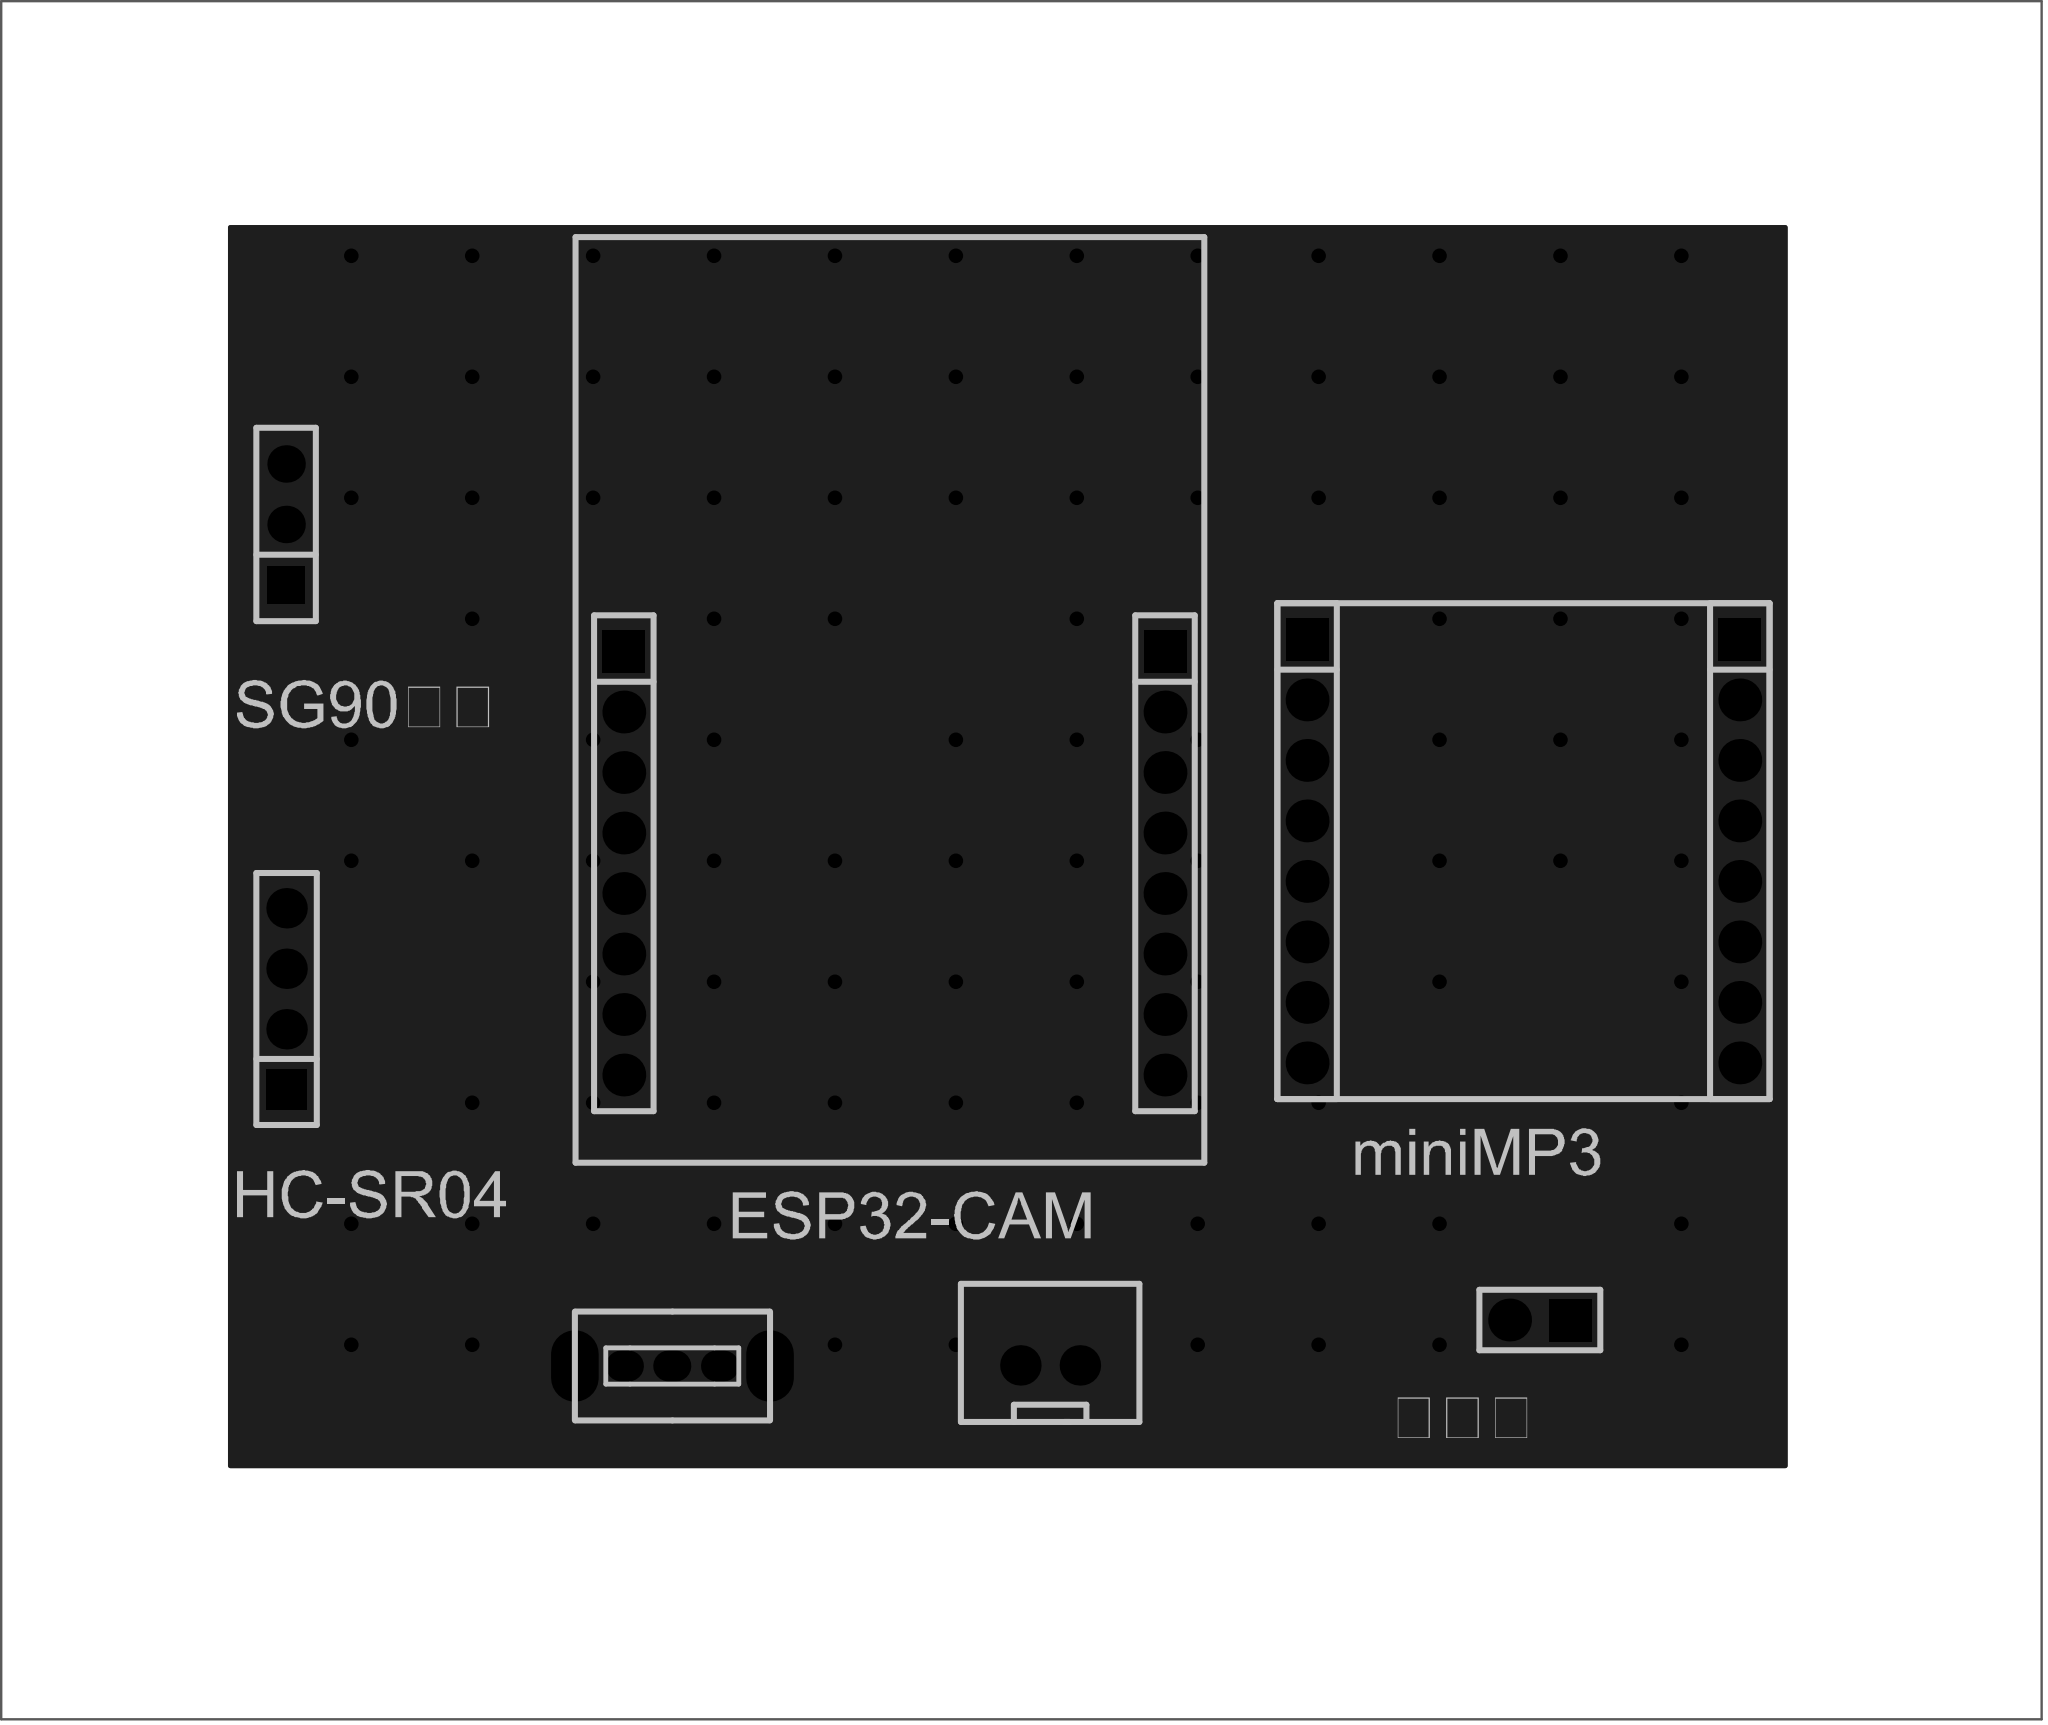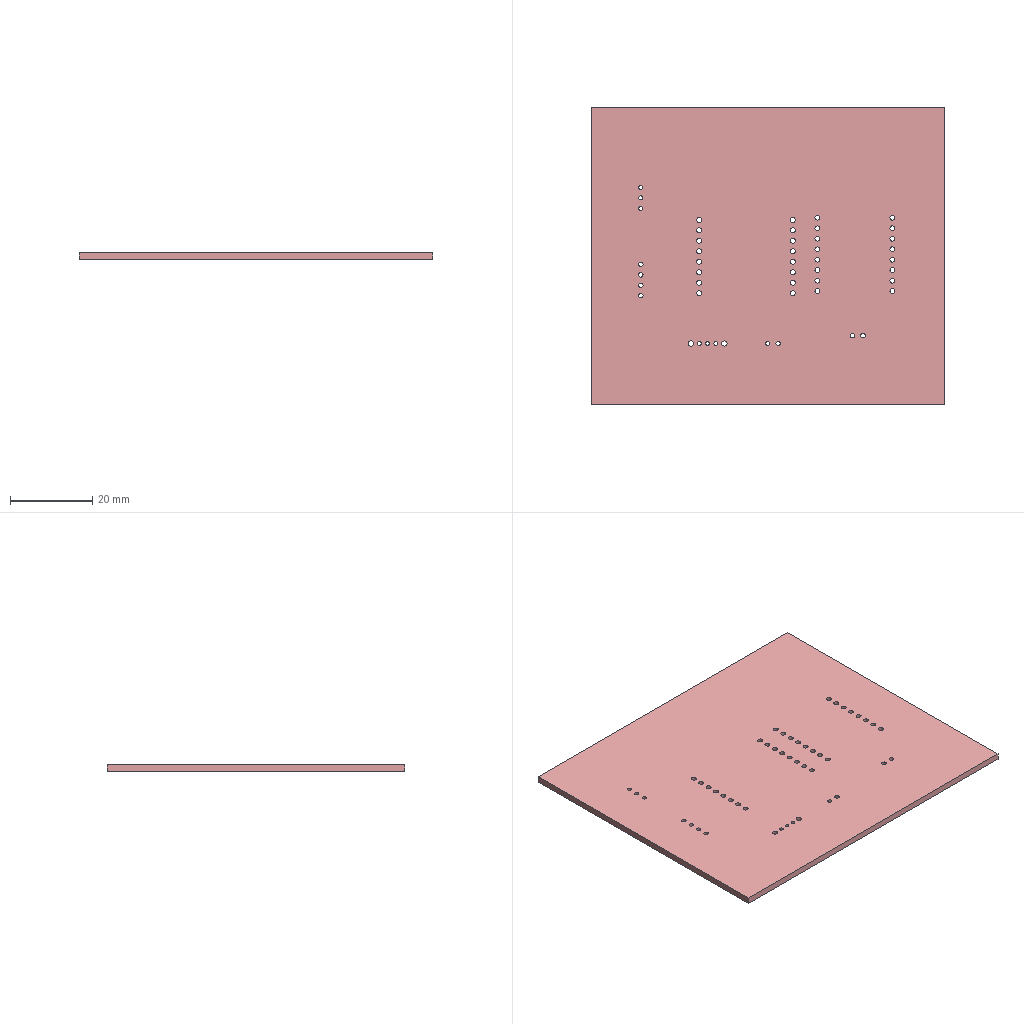Circuit board layout | Altium Designer | box 85.7 x 72.1 x 1.6 mm
Layer stack:
# Altium Designer layer stack of  (unit mm; dielectric type: 0 none, 1 core, 2 prepreg, 3 surface material)
index,name,kind,layer,copper_thickness_mm,dielectric_type,dielectric_thickness_mm,dielectric_material,dielectric_constant
0,Top Paste Mask Layer,other,,,,,,
1,Top Silkscreen Layer,other,,,,,,
2,Top Solder Mask Layer,dielectric,,,3,0.01,,3.3
3,Top Layer,copper,Top Layer,0.035,,,,
4,Dielectric1,dielectric,,,3,1.51,FR4,4.5
5,Bottom Layer,copper,Bottom Layer,0.035,,,,
6,Bottom Solder Mask Layer,dielectric,,,3,0.01,,3.3
7,Bottom Silkscreen Layer,other,,,,,,
8,Bottom Paste Mask Layer,other,,,,,,
# drill layer pairs: low layer,high layer
drill_pair,Top Layer,Bottom Layer
Part placement:
Designator,Comment,Layer,Footprint,Center-X(mm),Center-Y(mm),Rotation
CN4,XH2.54*2P_直插,TopLayer,CONN-TH_2P-P2.50-XH2.54-2P,113.919,84.709,180
H1,,TopLayer,HDR-TH_8P-P2.54-V-F-1,96.008,105.791,270
H2,,TopLayer,HDR-TH_8P-P2.54-V-F-1,118.745,105.791,270
H3,,TopLayer,HDR-TH_8P-P2.54-V-F-1,142.894,106.299,270
H4,,TopLayer,HDR-TH_8P-P2.54-V-F-1,124.714,106.299,270
H5,,TopLayer,HDR-TH_3P-P2.54-V-F,81.819,120.015,90
H6,,TopLayer,HDR-TH_2P-P2.54-V-M-1,134.493,86.614,180
H7,,TopLayer,HDR-TH_4P-P2.54-V-F,81.839,100.092,90
SW5,,TopLayer,拨动开关,98.052,84.683,0
Pad and via stacks:
# Altium Designer via and pad stacks of  (unit mm). Each distinct definition once, with the count of objects using it.
# via: kind,start_layer,end_layer,hole_mm,diameter_mm,mode(0 simple;1 top-mid-bottom;2 full stack),diameter_per_layer,count,example_net
# pad: kind,layer,hole_mm,hole_type(0 round;1 square;2 slot),plating,top_size,top_shape(1 round;2 rect;3 octagon;9 rounded rect),mid_size,bottom_size,mode,footprint,size_per_layer,count,example
pad,Multi-Layer,1.05,0,plated,1.7x1.7,1,1.7x1.7,1.7x1.7,0,CONN-TH_2P-P2.50-XH2.54-2P,,2,CN4.2
pad,Multi-Layer,1.2,0,plated,1.8x1.8,2,1.8x1.8,1.8x1.8,0,HDR-TH_8P-P2.54-V-F-1,,4,H1.1
pad,Multi-Layer,1.2,0,plated,1.8x1.8,1,1.8x1.8,1.8x1.8,0,HDR-TH_8P-P2.54-V-F-1,,28,H1.2
pad,Multi-Layer,1.02,0,plated,1.575x1.575,1,1.575x1.575,1.575x1.575,0,HDR-TH_3P-P2.54-V-F,,2,H5.3
pad,Multi-Layer,1.02,0,plated,1.575x1.575,2,1.575x1.575,1.575x1.575,0,HDR-TH_3P-P2.54-V-F,,1,H5.1
pad,Multi-Layer,1.1,0,plated,1.8x1.8,1,1.8x1.8,1.8x1.8,0,HDR-TH_2P-P2.54-V-M-1,,1,H6.2
pad,Multi-Layer,1.1,0,plated,1.8x1.8,2,1.8x1.8,1.8x1.8,0,HDR-TH_2P-P2.54-V-M-1,,1,H6.1
pad,Multi-Layer,1.1,0,plated,1.7x1.7,2,1.7x1.7,1.7x1.7,0,HDR-TH_4P-P2.54-V-F,,1,H7.1
pad,Multi-Layer,1.1,0,plated,1.7x1.7,1,1.7x1.7,1.7x1.7,0,HDR-TH_4P-P2.54-V-F,,3,H7.2
pad,Multi-Layer,0.8992,0,plated,1.6x1.3,1,1.6x1.3,1.6x1.3,0,\u00B2\u00A6\u00B6\u00AF\u00BF\u00AA\u00B9\u00D8,,3,SW5.1
pad,Multi-Layer,1.3,0,plated,3x1.999,1,3x1.999,3x1.999,0,\u00B2\u00A6\u00B6\u00AF\u00BF\u00AA\u00B9\u00D8,,2,SW5.4
via,Top Layer,Bottom Layer,0.3048,0.61,0,,99,GND
Copper pours:
name,layer,net,type(0 solid;1 hatched;2 none)
Bottom Layer-GND,Bottom Layer,GND,0
Top Layer-GND,Top Layer,GND,0